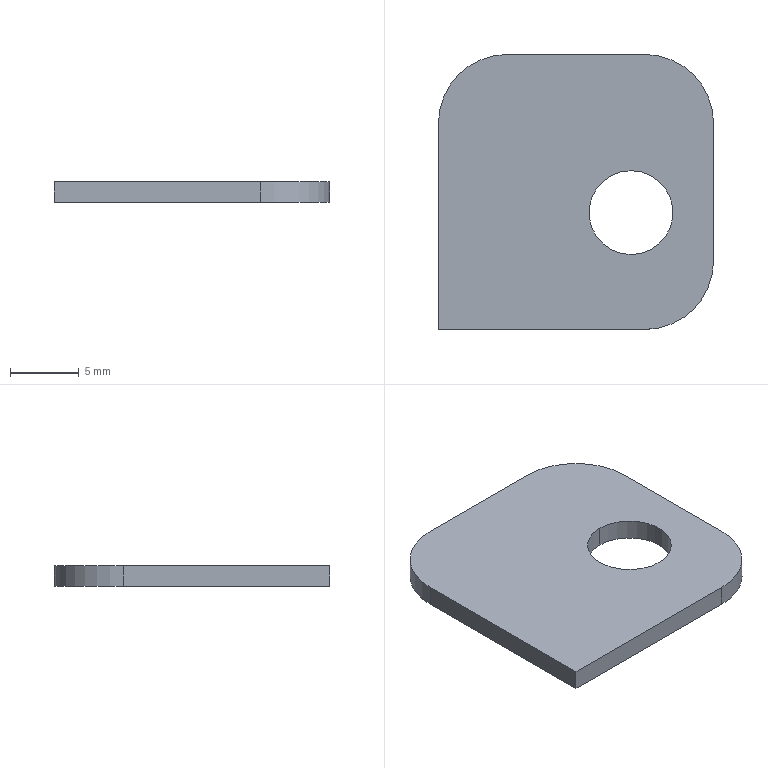Part | STEP file | 1 solid | 12 faces | box 20 x 20 x 1.5 mm | volume 532.02 mm3 | plane 7 | cylinder 5 | commonest cylinder face diameters 10 x3 6.1 x2
STEP:
#1=CARTESIAN_POINT('',(0.,0.,0.));
#2=DIRECTION('',(0.,0.,1.));
#3=DIRECTION('',(1.,0.,0.));
#4=AXIS2_PLACEMENT_3D('',#1,#2,#3);
#5=CARTESIAN_POINT('',(-500.773,4250.073,1738.644));
#6=VERTEX_POINT('',#5);
#7=CARTESIAN_POINT('',(-500.773,4256.573,1738.644));
#8=VERTEX_POINT('',#7);
#9=CARTESIAN_POINT('',(-500.773,4250.073,1738.644));
#10=DIRECTION('',(0.,1.,0.));
#11=VECTOR('',#10,1.);
#12=LINE('',#9,#11);
#13=CARTESIAN_POINT('',(-506.773,4250.073,1738.644));
#14=DIRECTION('',(0.,0.,-1.));
#15=DIRECTION('',(0.,-1.,0.));
#16=AXIS2_PLACEMENT_3D('',#13,#14,#15);
#17=PLANE('',#16);
#18=CARTESIAN_POINT('',(0.,-6.));
#19=DIRECTION('',(-1.,0.));
#20=VECTOR('',#19,1.);
#21=LINE('',#18,#20);
#22=(GEOMETRIC_REPRESENTATION_CONTEXT(2)PARAMETRIC_REPRESENTATION_CONTEXT()REPRESENTATION_CONTEXT('',''));
#23=DEFINITIONAL_REPRESENTATION('',(#21),#22);
#24=PCURVE('',#17,#23);
#25=CARTESIAN_POINT('',(-500.773,4255.823,1737.894));
#26=DIRECTION('',(-1.,0.,0.));
#27=DIRECTION('',(0.,-1.,0.));
#28=AXIS2_PLACEMENT_3D('',#25,#26,#27);
#29=PLANE('',#28);
#30=CARTESIAN_POINT('',(5.75,0.75));
#31=DIRECTION('',(-1.,0.));
#32=VECTOR('',#31,1.);
#33=LINE('',#30,#32);
#34=(GEOMETRIC_REPRESENTATION_CONTEXT(2)PARAMETRIC_REPRESENTATION_CONTEXT()REPRESENTATION_CONTEXT('',''));
#35=DEFINITIONAL_REPRESENTATION('',(#33),#34);
#36=PCURVE('',#29,#35);
#37=SURFACE_CURVE('',#12,(#24,#36),.PCURVE_S1.);
#38=EDGE_CURVE('',#6,#8,#37,.T.);
#39=ORIENTED_EDGE('',*,*,#38,.F.);
#40=CARTESIAN_POINT('',(-500.773,4246.573,1738.644));
#41=VERTEX_POINT('',#40);
#42=CARTESIAN_POINT('',(-500.773,4246.573,1738.644));
#43=DIRECTION('',(0.,1.,0.));
#44=VECTOR('',#43,1.);
#45=LINE('',#42,#44);
#46=CARTESIAN_POINT('',(3.5,-6.));
#47=DIRECTION('',(-1.,0.));
#48=VECTOR('',#47,1.);
#49=LINE('',#46,#48);
#50=(GEOMETRIC_REPRESENTATION_CONTEXT(2)PARAMETRIC_REPRESENTATION_CONTEXT()REPRESENTATION_CONTEXT('',''));
#51=DEFINITIONAL_REPRESENTATION('',(#49),#50);
#52=PCURVE('',#17,#51);
#53=CARTESIAN_POINT('',(-500.773,4245.823,1737.894));
#54=DIRECTION('',(-1.,0.,0.));
#55=DIRECTION('',(0.,-1.,0.));
#56=AXIS2_PLACEMENT_3D('',#53,#54,#55);
#57=PLANE('',#56);
#58=CARTESIAN_POINT('',(-0.75,0.75));
#59=DIRECTION('',(-1.,0.));
#60=VECTOR('',#59,1.);
#61=LINE('',#58,#60);
#62=(GEOMETRIC_REPRESENTATION_CONTEXT(2)PARAMETRIC_REPRESENTATION_CONTEXT()REPRESENTATION_CONTEXT('',''));
#63=DEFINITIONAL_REPRESENTATION('',(#61),#62);
#64=PCURVE('',#57,#63);
#65=SURFACE_CURVE('',#45,(#52,#64),.PCURVE_S1.);
#66=EDGE_CURVE('',#41,#6,#65,.T.);
#67=ORIENTED_EDGE('',*,*,#66,.F.);
#68=CARTESIAN_POINT('',(-505.773,4241.573,1738.644));
#69=VERTEX_POINT('',#68);
#70=CARTESIAN_POINT('',(-505.773,4246.573,1738.644));
#71=DIRECTION('',(0.,0.,1.));
#72=DIRECTION('',(0.,-1.,0.));
#73=AXIS2_PLACEMENT_3D('',#70,#71,#72);
#74=CIRCLE('',#73,5.);
#75=CARTESIAN_POINT('',(8.5,-1.));
#76=CARTESIAN_POINT('',(8.5,-9.66));
#77=CARTESIAN_POINT('',(1.,-5.33));
#78=CARTESIAN_POINT('',(-6.5,-1.));
#79=CARTESIAN_POINT('',(1.,3.33));
#80=CARTESIAN_POINT('',(8.5,7.66));
#81=CARTESIAN_POINT('',(8.5,-1.));
#82=(BOUNDED_CURVE()B_SPLINE_CURVE(2,(#75,#76,#77,#78,#79,#80,#81),.UNSPECIFIED.,.T.,.F.)B_SPLINE_CURVE_WITH_KNOTS((1,2,2,2,2,1),(-2.094,0.,2.094,4.189,6.283,8.378),.UNSPECIFIED.)CURVE()GEOMETRIC_REPRESENTATION_ITEM()RATIONAL_B_SPLINE_CURVE((1.,0.5,1.,0.5,1.,0.5,1.))REPRESENTATION_ITEM(''));
#83=(GEOMETRIC_REPRESENTATION_CONTEXT(2)PARAMETRIC_REPRESENTATION_CONTEXT()REPRESENTATION_CONTEXT('',''));
#84=DEFINITIONAL_REPRESENTATION('',(#82),#83);
#85=PCURVE('',#17,#84);
#86=CARTESIAN_POINT('',(-505.773,4246.573,1730.98));
#87=DIRECTION('',(0.,0.,1.));
#88=DIRECTION('',(-1.,0.,0.));
#89=AXIS2_PLACEMENT_3D('',#86,#87,#88);
#90=CYLINDRICAL_SURFACE('',#89,5.);
#91=CARTESIAN_POINT('',(1.571,7.664));
#92=DIRECTION('',(1.,0.));
#93=VECTOR('',#92,1.);
#94=LINE('',#91,#93);
#95=(GEOMETRIC_REPRESENTATION_CONTEXT(2)PARAMETRIC_REPRESENTATION_CONTEXT()REPRESENTATION_CONTEXT('',''));
#96=DEFINITIONAL_REPRESENTATION('',(#94),#95);
#97=PCURVE('',#90,#96);
#98=SURFACE_CURVE('',#74,(#85,#97),.PCURVE_S1.);
#99=EDGE_CURVE('',#69,#41,#98,.T.);
#100=ORIENTED_EDGE('',*,*,#99,.F.);
#101=CARTESIAN_POINT('',(-520.773,4241.573,1738.644));
#102=VERTEX_POINT('',#101);
#103=CARTESIAN_POINT('',(-520.773,4241.573,1738.644));
#104=DIRECTION('',(1.,0.,0.));
#105=VECTOR('',#104,1.);
#106=LINE('',#103,#105);
#107=CARTESIAN_POINT('',(8.5,14.));
#108=DIRECTION('',(0.,-1.));
#109=VECTOR('',#108,1.);
#110=LINE('',#107,#109);
#111=(GEOMETRIC_REPRESENTATION_CONTEXT(2)PARAMETRIC_REPRESENTATION_CONTEXT()REPRESENTATION_CONTEXT('',''));
#112=DEFINITIONAL_REPRESENTATION('',(#110),#111);
#113=PCURVE('',#17,#112);
#114=CARTESIAN_POINT('',(-510.773,4241.573,1737.894));
#115=DIRECTION('',(0.,1.,0.));
#116=DIRECTION('',(-1.,0.,0.));
#117=AXIS2_PLACEMENT_3D('',#114,#115,#116);
#118=PLANE('',#117);
#119=CARTESIAN_POINT('',(10.,0.75));
#120=DIRECTION('',(-1.,0.));
#121=VECTOR('',#120,1.);
#122=LINE('',#119,#121);
#123=(GEOMETRIC_REPRESENTATION_CONTEXT(2)PARAMETRIC_REPRESENTATION_CONTEXT()REPRESENTATION_CONTEXT('',''));
#124=DEFINITIONAL_REPRESENTATION('',(#122),#123);
#125=PCURVE('',#118,#124);
#126=SURFACE_CURVE('',#106,(#113,#125),.PCURVE_S1.);
#127=EDGE_CURVE('',#102,#69,#126,.T.);
#128=ORIENTED_EDGE('',*,*,#127,.F.);
#129=CARTESIAN_POINT('',(-520.773,4256.573,1738.644));
#130=VERTEX_POINT('',#129);
#131=CARTESIAN_POINT('',(-520.773,4256.573,1738.644));
#132=DIRECTION('',(0.,-1.,0.));
#133=VECTOR('',#132,1.);
#134=LINE('',#131,#133);
#135=CARTESIAN_POINT('',(-6.5,14.));
#136=DIRECTION('',(1.,0.));
#137=VECTOR('',#136,1.);
#138=LINE('',#135,#137);
#139=(GEOMETRIC_REPRESENTATION_CONTEXT(2)PARAMETRIC_REPRESENTATION_CONTEXT()REPRESENTATION_CONTEXT('',''));
#140=DEFINITIONAL_REPRESENTATION('',(#138),#139);
#141=PCURVE('',#17,#140);
#142=CARTESIAN_POINT('',(-520.773,4251.573,1737.894));
#143=DIRECTION('',(1.,0.,0.));
#144=DIRECTION('',(0.,1.,0.));
#145=AXIS2_PLACEMENT_3D('',#142,#143,#144);
#146=PLANE('',#145);
#147=CARTESIAN_POINT('',(5.,0.75));
#148=DIRECTION('',(-1.,0.));
#149=VECTOR('',#148,1.);
#150=LINE('',#147,#149);
#151=(GEOMETRIC_REPRESENTATION_CONTEXT(2)PARAMETRIC_REPRESENTATION_CONTEXT()REPRESENTATION_CONTEXT('',''));
#152=DEFINITIONAL_REPRESENTATION('',(#150),#151);
#153=PCURVE('',#146,#152);
#154=SURFACE_CURVE('',#134,(#141,#153),.PCURVE_S1.);
#155=EDGE_CURVE('',#130,#102,#154,.T.);
#156=ORIENTED_EDGE('',*,*,#155,.F.);
#157=CARTESIAN_POINT('',(-515.773,4261.573,1738.644));
#158=VERTEX_POINT('',#157);
#159=CARTESIAN_POINT('',(-515.773,4256.573,1738.644));
#160=DIRECTION('',(0.,0.,1.));
#161=DIRECTION('',(0.,1.,0.));
#162=AXIS2_PLACEMENT_3D('',#159,#160,#161);
#163=CIRCLE('',#162,5.);
#164=CARTESIAN_POINT('',(-11.5,9.));
#165=CARTESIAN_POINT('',(-11.5,17.66));
#166=CARTESIAN_POINT('',(-4.,13.33));
#167=CARTESIAN_POINT('',(3.5,9.));
#168=CARTESIAN_POINT('',(-4.,4.67));
#169=CARTESIAN_POINT('',(-11.5,0.3397));
#170=CARTESIAN_POINT('',(-11.5,9.));
#171=(BOUNDED_CURVE()B_SPLINE_CURVE(2,(#164,#165,#166,#167,#168,#169,#170),.UNSPECIFIED.,.T.,.F.)B_SPLINE_CURVE_WITH_KNOTS((1,2,2,2,2,1),(-2.094,0.,2.094,4.189,6.283,8.378),.UNSPECIFIED.)CURVE()GEOMETRIC_REPRESENTATION_ITEM()RATIONAL_B_SPLINE_CURVE((1.,0.5,1.,0.5,1.,0.5,1.))REPRESENTATION_ITEM(''));
#172=(GEOMETRIC_REPRESENTATION_CONTEXT(2)PARAMETRIC_REPRESENTATION_CONTEXT()REPRESENTATION_CONTEXT('',''));
#173=DEFINITIONAL_REPRESENTATION('',(#171),#172);
#174=PCURVE('',#17,#173);
#175=CARTESIAN_POINT('',(-515.773,4256.573,1730.98));
#176=DIRECTION('',(0.,0.,1.));
#177=DIRECTION('',(1.,0.,0.));
#178=AXIS2_PLACEMENT_3D('',#175,#176,#177);
#179=CYLINDRICAL_SURFACE('',#178,5.);
#180=CARTESIAN_POINT('',(1.571,7.664));
#181=DIRECTION('',(1.,0.));
#182=VECTOR('',#181,1.);
#183=LINE('',#180,#182);
#184=(GEOMETRIC_REPRESENTATION_CONTEXT(2)PARAMETRIC_REPRESENTATION_CONTEXT()REPRESENTATION_CONTEXT('',''));
#185=DEFINITIONAL_REPRESENTATION('',(#183),#184);
#186=PCURVE('',#179,#185);
#187=SURFACE_CURVE('',#163,(#174,#186),.PCURVE_S1.);
#188=EDGE_CURVE('',#158,#130,#187,.T.);
#189=ORIENTED_EDGE('',*,*,#188,.F.);
#190=CARTESIAN_POINT('',(-505.773,4261.573,1738.644));
#191=VERTEX_POINT('',#190);
#192=CARTESIAN_POINT('',(-505.773,4261.573,1738.644));
#193=DIRECTION('',(-1.,0.,0.));
#194=VECTOR('',#193,1.);
#195=LINE('',#192,#194);
#196=CARTESIAN_POINT('',(-11.5,-1.));
#197=DIRECTION('',(0.,1.));
#198=VECTOR('',#197,1.);
#199=LINE('',#196,#198);
#200=(GEOMETRIC_REPRESENTATION_CONTEXT(2)PARAMETRIC_REPRESENTATION_CONTEXT()REPRESENTATION_CONTEXT('',''));
#201=DEFINITIONAL_REPRESENTATION('',(#199),#200);
#202=PCURVE('',#17,#201);
#203=CARTESIAN_POINT('',(-510.773,4261.573,1737.894));
#204=DIRECTION('',(0.,-1.,0.));
#205=DIRECTION('',(1.,0.,0.));
#206=AXIS2_PLACEMENT_3D('',#203,#204,#205);
#207=PLANE('',#206);
#208=CARTESIAN_POINT('',(5.,0.75));
#209=DIRECTION('',(-1.,0.));
#210=VECTOR('',#209,1.);
#211=LINE('',#208,#210);
#212=(GEOMETRIC_REPRESENTATION_CONTEXT(2)PARAMETRIC_REPRESENTATION_CONTEXT()REPRESENTATION_CONTEXT('',''));
#213=DEFINITIONAL_REPRESENTATION('',(#211),#212);
#214=PCURVE('',#207,#213);
#215=SURFACE_CURVE('',#195,(#202,#214),.PCURVE_S1.);
#216=EDGE_CURVE('',#191,#158,#215,.T.);
#217=ORIENTED_EDGE('',*,*,#216,.F.);
#218=CARTESIAN_POINT('',(-505.773,4256.573,1738.644));
#219=DIRECTION('',(0.,0.,1.));
#220=DIRECTION('',(1.,0.,0.));
#221=AXIS2_PLACEMENT_3D('',#218,#219,#220);
#222=CIRCLE('',#221,5.);
#223=CARTESIAN_POINT('',(-6.5,-6.));
#224=CARTESIAN_POINT('',(-15.16,-6.));
#225=CARTESIAN_POINT('',(-10.83,1.5));
#226=CARTESIAN_POINT('',(-6.5,9.));
#227=CARTESIAN_POINT('',(-2.17,1.5));
#228=CARTESIAN_POINT('',(2.16,-6.));
#229=CARTESIAN_POINT('',(-6.5,-6.));
#230=(BOUNDED_CURVE()B_SPLINE_CURVE(2,(#223,#224,#225,#226,#227,#228,#229),.UNSPECIFIED.,.T.,.F.)B_SPLINE_CURVE_WITH_KNOTS((1,2,2,2,2,1),(-2.094,0.,2.094,4.189,6.283,8.378),.UNSPECIFIED.)CURVE()GEOMETRIC_REPRESENTATION_ITEM()RATIONAL_B_SPLINE_CURVE((1.,0.5,1.,0.5,1.,0.5,1.))REPRESENTATION_ITEM(''));
#231=(GEOMETRIC_REPRESENTATION_CONTEXT(2)PARAMETRIC_REPRESENTATION_CONTEXT()REPRESENTATION_CONTEXT('',''));
#232=DEFINITIONAL_REPRESENTATION('',(#230),#231);
#233=PCURVE('',#17,#232);
#234=CARTESIAN_POINT('',(-505.773,4256.573,1730.98));
#235=DIRECTION('',(0.,0.,1.));
#236=DIRECTION('',(0.,-1.,0.));
#237=AXIS2_PLACEMENT_3D('',#234,#235,#236);
#238=CYLINDRICAL_SURFACE('',#237,5.);
#239=CARTESIAN_POINT('',(1.571,7.664));
#240=DIRECTION('',(1.,0.));
#241=VECTOR('',#240,1.);
#242=LINE('',#239,#241);
#243=(GEOMETRIC_REPRESENTATION_CONTEXT(2)PARAMETRIC_REPRESENTATION_CONTEXT()REPRESENTATION_CONTEXT('',''));
#244=DEFINITIONAL_REPRESENTATION('',(#242),#243);
#245=PCURVE('',#238,#244);
#246=SURFACE_CURVE('',#222,(#233,#245),.PCURVE_S1.);
#247=EDGE_CURVE('',#8,#191,#246,.T.);
#248=ORIENTED_EDGE('',*,*,#247,.F.);
#249=EDGE_LOOP('',(#39,#67,#100,#128,#156,#189,#217,#248));
#250=FACE_BOUND('',#249,.F.);
#251=CARTESIAN_POINT('',(-506.773,4247.023,1738.644));
#252=VERTEX_POINT('',#251);
#253=CARTESIAN_POINT('',(-506.773,4253.123,1738.644));
#254=VERTEX_POINT('',#253);
#255=CARTESIAN_POINT('',(-506.773,4250.073,1738.644));
#256=DIRECTION('',(0.,0.,-1.));
#257=DIRECTION('',(0.,-1.,0.));
#258=AXIS2_PLACEMENT_3D('',#255,#256,#257);
#259=CIRCLE('',#258,3.05);
#260=CARTESIAN_POINT('',(0.,0.));
#261=DIRECTION('',(1.,0.));
#262=AXIS2_PLACEMENT_2D('',#260,#261);
#263=CIRCLE('',#262,3.05);
#264=(GEOMETRIC_REPRESENTATION_CONTEXT(2)PARAMETRIC_REPRESENTATION_CONTEXT()REPRESENTATION_CONTEXT('',''));
#265=DEFINITIONAL_REPRESENTATION('',(#263),#264);
#266=PCURVE('',#17,#265);
#267=CARTESIAN_POINT('',(-506.773,4250.073,1737.894));
#268=DIRECTION('',(0.,0.,1.));
#269=DIRECTION('',(0.,1.,0.));
#270=AXIS2_PLACEMENT_3D('',#267,#268,#269);
#271=CYLINDRICAL_SURFACE('',#270,3.05);
#272=CARTESIAN_POINT('',(3.142,0.75));
#273=DIRECTION('',(-1.,0.));
#274=VECTOR('',#273,1.);
#275=LINE('',#272,#274);
#276=(GEOMETRIC_REPRESENTATION_CONTEXT(2)PARAMETRIC_REPRESENTATION_CONTEXT()REPRESENTATION_CONTEXT('',''));
#277=DEFINITIONAL_REPRESENTATION('',(#275),#276);
#278=PCURVE('',#271,#277);
#279=SURFACE_CURVE('',#259,(#266,#278),.PCURVE_S1.);
#280=EDGE_CURVE('',#252,#254,#279,.T.);
#281=ORIENTED_EDGE('',*,*,#280,.F.);
#282=CARTESIAN_POINT('',(-506.773,4250.073,1738.644));
#283=DIRECTION('',(0.,0.,-1.));
#284=DIRECTION('',(0.,1.,0.));
#285=AXIS2_PLACEMENT_3D('',#282,#283,#284);
#286=CIRCLE('',#285,3.05);
#287=CARTESIAN_POINT('',(0.,0.));
#288=DIRECTION('',(-1.,0.));
#289=AXIS2_PLACEMENT_2D('',#287,#288);
#290=CIRCLE('',#289,3.05);
#291=(GEOMETRIC_REPRESENTATION_CONTEXT(2)PARAMETRIC_REPRESENTATION_CONTEXT()REPRESENTATION_CONTEXT('',''));
#292=DEFINITIONAL_REPRESENTATION('',(#290),#291);
#293=PCURVE('',#17,#292);
#294=CARTESIAN_POINT('',(-506.773,4250.073,1737.894));
#295=DIRECTION('',(0.,0.,1.));
#296=DIRECTION('',(0.,-1.,0.));
#297=AXIS2_PLACEMENT_3D('',#294,#295,#296);
#298=CYLINDRICAL_SURFACE('',#297,3.05);
#299=CARTESIAN_POINT('',(3.142,0.75));
#300=DIRECTION('',(-1.,0.));
#301=VECTOR('',#300,1.);
#302=LINE('',#299,#301);
#303=(GEOMETRIC_REPRESENTATION_CONTEXT(2)PARAMETRIC_REPRESENTATION_CONTEXT()REPRESENTATION_CONTEXT('',''));
#304=DEFINITIONAL_REPRESENTATION('',(#302),#303);
#305=PCURVE('',#298,#304);
#306=SURFACE_CURVE('',#286,(#293,#305),.PCURVE_S1.);
#307=EDGE_CURVE('',#254,#252,#306,.T.);
#308=ORIENTED_EDGE('',*,*,#307,.F.);
#309=EDGE_LOOP('',(#281,#308));
#310=FACE_BOUND('',#309,.F.);
#311=ADVANCED_FACE('',(#250,#310),#17,.F.);
#312=CARTESIAN_POINT('',(-500.773,4250.073,1737.144));
#313=VERTEX_POINT('',#312);
#314=CARTESIAN_POINT('',(-500.773,4256.573,1737.144));
#315=VERTEX_POINT('',#314);
#316=CARTESIAN_POINT('',(-500.773,4250.073,1737.144));
#317=DIRECTION('',(0.,1.,0.));
#318=VECTOR('',#317,1.);
#319=LINE('',#316,#318);
#320=CARTESIAN_POINT('',(5.75,-0.75));
#321=DIRECTION('',(-1.,0.));
#322=VECTOR('',#321,1.);
#323=LINE('',#320,#322);
#324=(GEOMETRIC_REPRESENTATION_CONTEXT(2)PARAMETRIC_REPRESENTATION_CONTEXT()REPRESENTATION_CONTEXT('',''));
#325=DEFINITIONAL_REPRESENTATION('',(#323),#324);
#326=PCURVE('',#29,#325);
#327=CARTESIAN_POINT('',(-506.773,4250.073,1737.144));
#328=DIRECTION('',(0.,0.,-1.));
#329=DIRECTION('',(0.,-1.,0.));
#330=AXIS2_PLACEMENT_3D('',#327,#328,#329);
#331=PLANE('',#330);
#332=CARTESIAN_POINT('',(0.,-6.));
#333=DIRECTION('',(-1.,0.));
#334=VECTOR('',#333,1.);
#335=LINE('',#332,#334);
#336=(GEOMETRIC_REPRESENTATION_CONTEXT(2)PARAMETRIC_REPRESENTATION_CONTEXT()REPRESENTATION_CONTEXT('',''));
#337=DEFINITIONAL_REPRESENTATION('',(#335),#336);
#338=PCURVE('',#331,#337);
#339=SURFACE_CURVE('',#319,(#326,#338),.PCURVE_S1.);
#340=EDGE_CURVE('',#313,#315,#339,.T.);
#341=ORIENTED_EDGE('',*,*,#340,.F.);
#342=CARTESIAN_POINT('',(-500.773,4250.073,1738.644));
#343=DIRECTION('',(0.,0.,-1.));
#344=VECTOR('',#343,1.);
#345=LINE('',#342,#344);
#346=CARTESIAN_POINT('',(5.75,0.75));
#347=DIRECTION('',(0.,-1.));
#348=VECTOR('',#347,1.);
#349=LINE('',#346,#348);
#350=(GEOMETRIC_REPRESENTATION_CONTEXT(2)PARAMETRIC_REPRESENTATION_CONTEXT()REPRESENTATION_CONTEXT('',''));
#351=DEFINITIONAL_REPRESENTATION('',(#349),#350);
#352=PCURVE('',#29,#351);
#353=CARTESIAN_POINT('',(-4.25,0.75));
#354=DIRECTION('',(0.,-1.));
#355=VECTOR('',#354,1.);
#356=LINE('',#353,#355);
#357=(GEOMETRIC_REPRESENTATION_CONTEXT(2)PARAMETRIC_REPRESENTATION_CONTEXT()REPRESENTATION_CONTEXT('',''));
#358=DEFINITIONAL_REPRESENTATION('',(#356),#357);
#359=PCURVE('',#57,#358);
#360=SURFACE_CURVE('',#345,(#352,#359),.PCURVE_S1.);
#361=EDGE_CURVE('',#6,#313,#360,.T.);
#362=ORIENTED_EDGE('',*,*,#361,.F.);
#363=ORIENTED_EDGE('',*,*,#38,.T.);
#364=CARTESIAN_POINT('',(-500.773,4256.573,1738.644));
#365=DIRECTION('',(0.,0.,-1.));
#366=VECTOR('',#365,1.);
#367=LINE('',#364,#366);
#368=CARTESIAN_POINT('',(-0.75,0.75));
#369=DIRECTION('',(0.,-1.));
#370=VECTOR('',#369,1.);
#371=LINE('',#368,#370);
#372=(GEOMETRIC_REPRESENTATION_CONTEXT(2)PARAMETRIC_REPRESENTATION_CONTEXT()REPRESENTATION_CONTEXT('',''));
#373=DEFINITIONAL_REPRESENTATION('',(#371),#372);
#374=PCURVE('',#29,#373);
#375=CARTESIAN_POINT('',(1.571,7.664));
#376=DIRECTION('',(0.,-1.));
#377=VECTOR('',#376,1.);
#378=LINE('',#375,#377);
#379=(GEOMETRIC_REPRESENTATION_CONTEXT(2)PARAMETRIC_REPRESENTATION_CONTEXT()REPRESENTATION_CONTEXT('',''));
#380=DEFINITIONAL_REPRESENTATION('',(#378),#379);
#381=PCURVE('',#238,#380);
#382=SURFACE_CURVE('',#367,(#374,#381),.PCURVE_S1.);
#383=EDGE_CURVE('',#8,#315,#382,.T.);
#384=ORIENTED_EDGE('',*,*,#383,.T.);
#385=EDGE_LOOP('',(#341,#362,#363,#384));
#386=FACE_BOUND('',#385,.F.);
#387=ADVANCED_FACE('',(#386),#29,.F.);
#388=CARTESIAN_POINT('',(-505.773,4261.573,1737.144));
#389=VERTEX_POINT('',#388);
#390=CARTESIAN_POINT('',(-515.773,4261.573,1737.144));
#391=VERTEX_POINT('',#390);
#392=CARTESIAN_POINT('',(-505.773,4261.573,1737.144));
#393=DIRECTION('',(-1.,0.,0.));
#394=VECTOR('',#393,1.);
#395=LINE('',#392,#394);
#396=CARTESIAN_POINT('',(-11.5,-1.));
#397=DIRECTION('',(0.,1.));
#398=VECTOR('',#397,1.);
#399=LINE('',#396,#398);
#400=(GEOMETRIC_REPRESENTATION_CONTEXT(2)PARAMETRIC_REPRESENTATION_CONTEXT()REPRESENTATION_CONTEXT('',''));
#401=DEFINITIONAL_REPRESENTATION('',(#399),#400);
#402=PCURVE('',#331,#401);
#403=CARTESIAN_POINT('',(5.,-0.75));
#404=DIRECTION('',(-1.,0.));
#405=VECTOR('',#404,1.);
#406=LINE('',#403,#405);
#407=(GEOMETRIC_REPRESENTATION_CONTEXT(2)PARAMETRIC_REPRESENTATION_CONTEXT()REPRESENTATION_CONTEXT('',''));
#408=DEFINITIONAL_REPRESENTATION('',(#406),#407);
#409=PCURVE('',#207,#408);
#410=SURFACE_CURVE('',#395,(#402,#409),.PCURVE_S1.);
#411=EDGE_CURVE('',#389,#391,#410,.T.);
#412=ORIENTED_EDGE('',*,*,#411,.T.);
#413=CARTESIAN_POINT('',(-520.773,4256.573,1737.144));
#414=VERTEX_POINT('',#413);
#415=CARTESIAN_POINT('',(-515.773,4256.573,1737.144));
#416=DIRECTION('',(0.,0.,-1.));
#417=DIRECTION('',(-1.,0.,0.));
#418=AXIS2_PLACEMENT_3D('',#415,#416,#417);
#419=CIRCLE('',#418,5.);
#420=CARTESIAN_POINT('',(-6.5,9.));
#421=DIRECTION('',(0.,1.));
#422=AXIS2_PLACEMENT_2D('',#420,#421);
#423=CIRCLE('',#422,5.);
#424=(GEOMETRIC_REPRESENTATION_CONTEXT(2)PARAMETRIC_REPRESENTATION_CONTEXT()REPRESENTATION_CONTEXT('',''));
#425=DEFINITIONAL_REPRESENTATION('',(#423),#424);
#426=PCURVE('',#331,#425);
#427=CARTESIAN_POINT('',(3.142,6.164));
#428=DIRECTION('',(-1.,0.));
#429=VECTOR('',#428,1.);
#430=LINE('',#427,#429);
#431=(GEOMETRIC_REPRESENTATION_CONTEXT(2)PARAMETRIC_REPRESENTATION_CONTEXT()REPRESENTATION_CONTEXT('',''));
#432=DEFINITIONAL_REPRESENTATION('',(#430),#431);
#433=PCURVE('',#179,#432);
#434=SURFACE_CURVE('',#419,(#426,#433),.PCURVE_S1.);
#435=EDGE_CURVE('',#414,#391,#434,.T.);
#436=ORIENTED_EDGE('',*,*,#435,.F.);
#437=CARTESIAN_POINT('',(-520.773,4241.573,1737.144));
#438=VERTEX_POINT('',#437);
#439=CARTESIAN_POINT('',(-520.773,4256.573,1737.144));
#440=DIRECTION('',(0.,-1.,0.));
#441=VECTOR('',#440,1.);
#442=LINE('',#439,#441);
#443=CARTESIAN_POINT('',(-6.5,14.));
#444=DIRECTION('',(1.,0.));
#445=VECTOR('',#444,1.);
#446=LINE('',#443,#445);
#447=(GEOMETRIC_REPRESENTATION_CONTEXT(2)PARAMETRIC_REPRESENTATION_CONTEXT()REPRESENTATION_CONTEXT('',''));
#448=DEFINITIONAL_REPRESENTATION('',(#446),#447);
#449=PCURVE('',#331,#448);
#450=CARTESIAN_POINT('',(5.,-0.75));
#451=DIRECTION('',(-1.,0.));
#452=VECTOR('',#451,1.);
#453=LINE('',#450,#452);
#454=(GEOMETRIC_REPRESENTATION_CONTEXT(2)PARAMETRIC_REPRESENTATION_CONTEXT()REPRESENTATION_CONTEXT('',''));
#455=DEFINITIONAL_REPRESENTATION('',(#453),#454);
#456=PCURVE('',#146,#455);
#457=SURFACE_CURVE('',#442,(#449,#456),.PCURVE_S1.);
#458=EDGE_CURVE('',#414,#438,#457,.T.);
#459=ORIENTED_EDGE('',*,*,#458,.T.);
#460=CARTESIAN_POINT('',(-505.773,4241.573,1737.144));
#461=VERTEX_POINT('',#460);
#462=CARTESIAN_POINT('',(-520.773,4241.573,1737.144));
#463=DIRECTION('',(1.,0.,0.));
#464=VECTOR('',#463,1.);
#465=LINE('',#462,#464);
#466=CARTESIAN_POINT('',(8.5,14.));
#467=DIRECTION('',(0.,-1.));
#468=VECTOR('',#467,1.);
#469=LINE('',#466,#468);
#470=(GEOMETRIC_REPRESENTATION_CONTEXT(2)PARAMETRIC_REPRESENTATION_CONTEXT()REPRESENTATION_CONTEXT('',''));
#471=DEFINITIONAL_REPRESENTATION('',(#469),#470);
#472=PCURVE('',#331,#471);
#473=CARTESIAN_POINT('',(10.,-0.75));
#474=DIRECTION('',(-1.,0.));
#475=VECTOR('',#474,1.);
#476=LINE('',#473,#475);
#477=(GEOMETRIC_REPRESENTATION_CONTEXT(2)PARAMETRIC_REPRESENTATION_CONTEXT()REPRESENTATION_CONTEXT('',''));
#478=DEFINITIONAL_REPRESENTATION('',(#476),#477);
#479=PCURVE('',#118,#478);
#480=SURFACE_CURVE('',#465,(#472,#479),.PCURVE_S1.);
#481=EDGE_CURVE('',#438,#461,#480,.T.);
#482=ORIENTED_EDGE('',*,*,#481,.T.);
#483=CARTESIAN_POINT('',(-500.773,4246.573,1737.144));
#484=VERTEX_POINT('',#483);
#485=CARTESIAN_POINT('',(-505.773,4246.573,1737.144));
#486=DIRECTION('',(0.,0.,-1.));
#487=DIRECTION('',(1.,0.,0.));
#488=AXIS2_PLACEMENT_3D('',#485,#486,#487);
#489=CIRCLE('',#488,5.);
#490=CARTESIAN_POINT('',(3.5,-1.));
#491=DIRECTION('',(0.,-1.));
#492=AXIS2_PLACEMENT_2D('',#490,#491);
#493=CIRCLE('',#492,5.);
#494=(GEOMETRIC_REPRESENTATION_CONTEXT(2)PARAMETRIC_REPRESENTATION_CONTEXT()REPRESENTATION_CONTEXT('',''));
#495=DEFINITIONAL_REPRESENTATION('',(#493),#494);
#496=PCURVE('',#331,#495);
#497=CARTESIAN_POINT('',(3.142,6.164));
#498=DIRECTION('',(-1.,0.));
#499=VECTOR('',#498,1.);
#500=LINE('',#497,#499);
#501=(GEOMETRIC_REPRESENTATION_CONTEXT(2)PARAMETRIC_REPRESENTATION_CONTEXT()REPRESENTATION_CONTEXT('',''));
#502=DEFINITIONAL_REPRESENTATION('',(#500),#501);
#503=PCURVE('',#90,#502);
#504=SURFACE_CURVE('',#489,(#496,#503),.PCURVE_S1.);
#505=EDGE_CURVE('',#484,#461,#504,.T.);
#506=ORIENTED_EDGE('',*,*,#505,.F.);
#507=CARTESIAN_POINT('',(-500.773,4246.573,1737.144));
#508=DIRECTION('',(0.,1.,0.));
#509=VECTOR('',#508,1.);
#510=LINE('',#507,#509);
#511=CARTESIAN_POINT('',(3.5,-6.));
#512=DIRECTION('',(-1.,0.));
#513=VECTOR('',#512,1.);
#514=LINE('',#511,#513);
#515=(GEOMETRIC_REPRESENTATION_CONTEXT(2)PARAMETRIC_REPRESENTATION_CONTEXT()REPRESENTATION_CONTEXT('',''));
#516=DEFINITIONAL_REPRESENTATION('',(#514),#515);
#517=PCURVE('',#331,#516);
#518=CARTESIAN_POINT('',(-0.75,-0.75));
#519=DIRECTION('',(-1.,0.));
#520=VECTOR('',#519,1.);
#521=LINE('',#518,#520);
#522=(GEOMETRIC_REPRESENTATION_CONTEXT(2)PARAMETRIC_REPRESENTATION_CONTEXT()REPRESENTATION_CONTEXT('',''));
#523=DEFINITIONAL_REPRESENTATION('',(#521),#522);
#524=PCURVE('',#57,#523);
#525=SURFACE_CURVE('',#510,(#517,#524),.PCURVE_S1.);
#526=EDGE_CURVE('',#484,#313,#525,.T.);
#527=ORIENTED_EDGE('',*,*,#526,.T.);
#528=ORIENTED_EDGE('',*,*,#340,.T.);
#529=CARTESIAN_POINT('',(-505.773,4256.573,1737.144));
#530=DIRECTION('',(0.,0.,-1.));
#531=DIRECTION('',(0.,1.,0.));
#532=AXIS2_PLACEMENT_3D('',#529,#530,#531);
#533=CIRCLE('',#532,5.);
#534=CARTESIAN_POINT('',(-6.5,-1.));
#535=DIRECTION('',(-1.,0.));
#536=AXIS2_PLACEMENT_2D('',#534,#535);
#537=CIRCLE('',#536,5.);
#538=(GEOMETRIC_REPRESENTATION_CONTEXT(2)PARAMETRIC_REPRESENTATION_CONTEXT()REPRESENTATION_CONTEXT('',''));
#539=DEFINITIONAL_REPRESENTATION('',(#537),#538);
#540=PCURVE('',#331,#539);
#541=CARTESIAN_POINT('',(3.142,6.164));
#542=DIRECTION('',(-1.,0.));
#543=VECTOR('',#542,1.);
#544=LINE('',#541,#543);
#545=(GEOMETRIC_REPRESENTATION_CONTEXT(2)PARAMETRIC_REPRESENTATION_CONTEXT()REPRESENTATION_CONTEXT('',''));
#546=DEFINITIONAL_REPRESENTATION('',(#544),#545);
#547=PCURVE('',#238,#546);
#548=SURFACE_CURVE('',#533,(#540,#547),.PCURVE_S1.);
#549=EDGE_CURVE('',#389,#315,#548,.T.);
#550=ORIENTED_EDGE('',*,*,#549,.F.);
#551=EDGE_LOOP('',(#412,#436,#459,#482,#506,#527,#528,#550));
#552=FACE_BOUND('',#551,.F.);
#553=CARTESIAN_POINT('',(-506.773,4253.123,1737.144));
#554=VERTEX_POINT('',#553);
#555=CARTESIAN_POINT('',(-506.773,4247.023,1737.144));
#556=VERTEX_POINT('',#555);
#557=CARTESIAN_POINT('',(-506.773,4250.073,1737.144));
#558=DIRECTION('',(0.,0.,1.));
#559=DIRECTION('',(0.,1.,0.));
#560=AXIS2_PLACEMENT_3D('',#557,#558,#559);
#561=CIRCLE('',#560,3.05);
#562=CARTESIAN_POINT('',(-3.05,0.));
#563=CARTESIAN_POINT('',(-3.05,5.283));
#564=CARTESIAN_POINT('',(1.525,2.641));
#565=CARTESIAN_POINT('',(6.1,0.));
#566=CARTESIAN_POINT('',(1.525,-2.641));
#567=CARTESIAN_POINT('',(-3.05,-5.283));
#568=CARTESIAN_POINT('',(-3.05,0.));
#569=(BOUNDED_CURVE()B_SPLINE_CURVE(2,(#562,#563,#564,#565,#566,#567,#568),.UNSPECIFIED.,.T.,.F.)B_SPLINE_CURVE_WITH_KNOTS((1,2,2,2,2,1),(-2.094,0.,2.094,4.189,6.283,8.378),.UNSPECIFIED.)CURVE()GEOMETRIC_REPRESENTATION_ITEM()RATIONAL_B_SPLINE_CURVE((1.,0.5,1.,0.5,1.,0.5,1.))REPRESENTATION_ITEM(''));
#570=(GEOMETRIC_REPRESENTATION_CONTEXT(2)PARAMETRIC_REPRESENTATION_CONTEXT()REPRESENTATION_CONTEXT('',''));
#571=DEFINITIONAL_REPRESENTATION('',(#569),#570);
#572=PCURVE('',#331,#571);
#573=CARTESIAN_POINT('',(0.,-0.75));
#574=DIRECTION('',(1.,0.));
#575=VECTOR('',#574,1.);
#576=LINE('',#573,#575);
#577=(GEOMETRIC_REPRESENTATION_CONTEXT(2)PARAMETRIC_REPRESENTATION_CONTEXT()REPRESENTATION_CONTEXT('',''));
#578=DEFINITIONAL_REPRESENTATION('',(#576),#577);
#579=PCURVE('',#271,#578);
#580=SURFACE_CURVE('',#561,(#572,#579),.PCURVE_S1.);
#581=EDGE_CURVE('',#554,#556,#580,.T.);
#582=ORIENTED_EDGE('',*,*,#581,.F.);
#583=CARTESIAN_POINT('',(-506.773,4250.073,1737.144));
#584=DIRECTION('',(0.,0.,1.));
#585=DIRECTION('',(0.,-1.,0.));
#586=AXIS2_PLACEMENT_3D('',#583,#584,#585);
#587=CIRCLE('',#586,3.05);
#588=CARTESIAN_POINT('',(3.05,0.));
#589=CARTESIAN_POINT('',(3.05,-5.283));
#590=CARTESIAN_POINT('',(-1.525,-2.641));
#591=CARTESIAN_POINT('',(-6.1,0.));
#592=CARTESIAN_POINT('',(-1.525,2.641));
#593=CARTESIAN_POINT('',(3.05,5.283));
#594=CARTESIAN_POINT('',(3.05,0.));
#595=(BOUNDED_CURVE()B_SPLINE_CURVE(2,(#588,#589,#590,#591,#592,#593,#594),.UNSPECIFIED.,.T.,.F.)B_SPLINE_CURVE_WITH_KNOTS((1,2,2,2,2,1),(-2.094,0.,2.094,4.189,6.283,8.378),.UNSPECIFIED.)CURVE()GEOMETRIC_REPRESENTATION_ITEM()RATIONAL_B_SPLINE_CURVE((1.,0.5,1.,0.5,1.,0.5,1.))REPRESENTATION_ITEM(''));
#596=(GEOMETRIC_REPRESENTATION_CONTEXT(2)PARAMETRIC_REPRESENTATION_CONTEXT()REPRESENTATION_CONTEXT('',''));
#597=DEFINITIONAL_REPRESENTATION('',(#595),#596);
#598=PCURVE('',#331,#597);
#599=CARTESIAN_POINT('',(0.,-0.75));
#600=DIRECTION('',(1.,0.));
#601=VECTOR('',#600,1.);
#602=LINE('',#599,#601);
#603=(GEOMETRIC_REPRESENTATION_CONTEXT(2)PARAMETRIC_REPRESENTATION_CONTEXT()REPRESENTATION_CONTEXT('',''));
#604=DEFINITIONAL_REPRESENTATION('',(#602),#603);
#605=PCURVE('',#298,#604);
#606=SURFACE_CURVE('',#587,(#598,#605),.PCURVE_S1.);
#607=EDGE_CURVE('',#556,#554,#606,.T.);
#608=ORIENTED_EDGE('',*,*,#607,.F.);
#609=EDGE_LOOP('',(#582,#608));
#610=FACE_BOUND('',#609,.F.);
#611=ADVANCED_FACE('',(#552,#610),#331,.T.);
#612=ORIENTED_EDGE('',*,*,#216,.T.);
#613=CARTESIAN_POINT('',(-515.773,4261.573,1738.644));
#614=DIRECTION('',(0.,0.,-1.));
#615=VECTOR('',#614,1.);
#616=LINE('',#613,#615);
#617=CARTESIAN_POINT('',(-5.,0.75));
#618=DIRECTION('',(0.,-1.));
#619=VECTOR('',#618,1.);
#620=LINE('',#617,#619);
#621=(GEOMETRIC_REPRESENTATION_CONTEXT(2)PARAMETRIC_REPRESENTATION_CONTEXT()REPRESENTATION_CONTEXT('',''));
#622=DEFINITIONAL_REPRESENTATION('',(#620),#621);
#623=PCURVE('',#207,#622);
#624=CARTESIAN_POINT('',(1.571,7.664));
#625=DIRECTION('',(0.,-1.));
#626=VECTOR('',#625,1.);
#627=LINE('',#624,#626);
#628=(GEOMETRIC_REPRESENTATION_CONTEXT(2)PARAMETRIC_REPRESENTATION_CONTEXT()REPRESENTATION_CONTEXT('',''));
#629=DEFINITIONAL_REPRESENTATION('',(#627),#628);
#630=PCURVE('',#179,#629);
#631=SURFACE_CURVE('',#616,(#623,#630),.PCURVE_S1.);
#632=EDGE_CURVE('',#158,#391,#631,.T.);
#633=ORIENTED_EDGE('',*,*,#632,.T.);
#634=ORIENTED_EDGE('',*,*,#411,.F.);
#635=CARTESIAN_POINT('',(-505.773,4261.573,1737.144));
#636=DIRECTION('',(0.,0.,1.));
#637=VECTOR('',#636,1.);
#638=LINE('',#635,#637);
#639=CARTESIAN_POINT('',(5.,-0.75));
#640=DIRECTION('',(0.,1.));
#641=VECTOR('',#640,1.);
#642=LINE('',#639,#641);
#643=(GEOMETRIC_REPRESENTATION_CONTEXT(2)PARAMETRIC_REPRESENTATION_CONTEXT()REPRESENTATION_CONTEXT('',''));
#644=DEFINITIONAL_REPRESENTATION('',(#642),#643);
#645=PCURVE('',#207,#644);
#646=CARTESIAN_POINT('',(3.142,6.164));
#647=DIRECTION('',(0.,1.));
#648=VECTOR('',#647,1.);
#649=LINE('',#646,#648);
#650=(GEOMETRIC_REPRESENTATION_CONTEXT(2)PARAMETRIC_REPRESENTATION_CONTEXT()REPRESENTATION_CONTEXT('',''));
#651=DEFINITIONAL_REPRESENTATION('',(#649),#650);
#652=PCURVE('',#238,#651);
#653=SURFACE_CURVE('',#638,(#645,#652),.PCURVE_S1.);
#654=EDGE_CURVE('',#389,#191,#653,.T.);
#655=ORIENTED_EDGE('',*,*,#654,.T.);
#656=EDGE_LOOP('',(#612,#633,#634,#655));
#657=FACE_BOUND('',#656,.F.);
#658=ADVANCED_FACE('',(#657),#207,.F.);
#659=ORIENTED_EDGE('',*,*,#188,.F.);
#660=ORIENTED_EDGE('',*,*,#632,.T.);
#661=ORIENTED_EDGE('',*,*,#435,.F.);
#662=CARTESIAN_POINT('',(-520.773,4256.573,1737.144));
#663=DIRECTION('',(0.,0.,1.));
#664=VECTOR('',#663,1.);
#665=LINE('',#662,#664);
#666=CARTESIAN_POINT('',(3.142,6.164));
#667=DIRECTION('',(0.,1.));
#668=VECTOR('',#667,1.);
#669=LINE('',#666,#668);
#670=(GEOMETRIC_REPRESENTATION_CONTEXT(2)PARAMETRIC_REPRESENTATION_CONTEXT()REPRESENTATION_CONTEXT('',''));
#671=DEFINITIONAL_REPRESENTATION('',(#669),#670);
#672=PCURVE('',#179,#671);
#673=CARTESIAN_POINT('',(5.,-0.75));
#674=DIRECTION('',(0.,1.));
#675=VECTOR('',#674,1.);
#676=LINE('',#673,#675);
#677=(GEOMETRIC_REPRESENTATION_CONTEXT(2)PARAMETRIC_REPRESENTATION_CONTEXT()REPRESENTATION_CONTEXT('',''));
#678=DEFINITIONAL_REPRESENTATION('',(#676),#677);
#679=PCURVE('',#146,#678);
#680=SURFACE_CURVE('',#665,(#672,#679),.PCURVE_S1.);
#681=EDGE_CURVE('',#414,#130,#680,.T.);
#682=ORIENTED_EDGE('',*,*,#681,.T.);
#683=EDGE_LOOP('',(#659,#660,#661,#682));
#684=FACE_BOUND('',#683,.T.);
#685=ADVANCED_FACE('',(#684),#179,.T.);
#686=ORIENTED_EDGE('',*,*,#155,.T.);
#687=CARTESIAN_POINT('',(-520.773,4241.573,1738.644));
#688=DIRECTION('',(0.,0.,-1.));
#689=VECTOR('',#688,1.);
#690=LINE('',#687,#689);
#691=CARTESIAN_POINT('',(-10.,0.75));
#692=DIRECTION('',(0.,-1.));
#693=VECTOR('',#692,1.);
#694=LINE('',#691,#693);
#695=(GEOMETRIC_REPRESENTATION_CONTEXT(2)PARAMETRIC_REPRESENTATION_CONTEXT()REPRESENTATION_CONTEXT('',''));
#696=DEFINITIONAL_REPRESENTATION('',(#694),#695);
#697=PCURVE('',#146,#696);
#698=CARTESIAN_POINT('',(10.,0.75));
#699=DIRECTION('',(0.,-1.));
#700=VECTOR('',#699,1.);
#701=LINE('',#698,#700);
#702=(GEOMETRIC_REPRESENTATION_CONTEXT(2)PARAMETRIC_REPRESENTATION_CONTEXT()REPRESENTATION_CONTEXT('',''));
#703=DEFINITIONAL_REPRESENTATION('',(#701),#702);
#704=PCURVE('',#118,#703);
#705=SURFACE_CURVE('',#690,(#697,#704),.PCURVE_S1.);
#706=EDGE_CURVE('',#102,#438,#705,.T.);
#707=ORIENTED_EDGE('',*,*,#706,.T.);
#708=ORIENTED_EDGE('',*,*,#458,.F.);
#709=ORIENTED_EDGE('',*,*,#681,.T.);
#710=EDGE_LOOP('',(#686,#707,#708,#709));
#711=FACE_BOUND('',#710,.F.);
#712=ADVANCED_FACE('',(#711),#146,.F.);
#713=ORIENTED_EDGE('',*,*,#481,.F.);
#714=ORIENTED_EDGE('',*,*,#706,.F.);
#715=ORIENTED_EDGE('',*,*,#127,.T.);
#716=CARTESIAN_POINT('',(-505.773,4241.573,1738.644));
#717=DIRECTION('',(0.,0.,-1.));
#718=VECTOR('',#717,1.);
#719=LINE('',#716,#718);
#720=CARTESIAN_POINT('',(-5.,0.75));
#721=DIRECTION('',(0.,-1.));
#722=VECTOR('',#721,1.);
#723=LINE('',#720,#722);
#724=(GEOMETRIC_REPRESENTATION_CONTEXT(2)PARAMETRIC_REPRESENTATION_CONTEXT()REPRESENTATION_CONTEXT('',''));
#725=DEFINITIONAL_REPRESENTATION('',(#723),#724);
#726=PCURVE('',#118,#725);
#727=CARTESIAN_POINT('',(1.571,7.664));
#728=DIRECTION('',(0.,-1.));
#729=VECTOR('',#728,1.);
#730=LINE('',#727,#729);
#731=(GEOMETRIC_REPRESENTATION_CONTEXT(2)PARAMETRIC_REPRESENTATION_CONTEXT()REPRESENTATION_CONTEXT('',''));
#732=DEFINITIONAL_REPRESENTATION('',(#730),#731);
#733=PCURVE('',#90,#732);
#734=SURFACE_CURVE('',#719,(#726,#733),.PCURVE_S1.);
#735=EDGE_CURVE('',#69,#461,#734,.T.);
#736=ORIENTED_EDGE('',*,*,#735,.T.);
#737=EDGE_LOOP('',(#713,#714,#715,#736));
#738=FACE_BOUND('',#737,.F.);
#739=ADVANCED_FACE('',(#738),#118,.F.);
#740=ORIENTED_EDGE('',*,*,#99,.F.);
#741=ORIENTED_EDGE('',*,*,#735,.T.);
#742=ORIENTED_EDGE('',*,*,#505,.F.);
#743=CARTESIAN_POINT('',(-500.773,4246.573,1737.144));
#744=DIRECTION('',(0.,0.,1.));
#745=VECTOR('',#744,1.);
#746=LINE('',#743,#745);
#747=CARTESIAN_POINT('',(3.142,6.164));
#748=DIRECTION('',(0.,1.));
#749=VECTOR('',#748,1.);
#750=LINE('',#747,#749);
#751=(GEOMETRIC_REPRESENTATION_CONTEXT(2)PARAMETRIC_REPRESENTATION_CONTEXT()REPRESENTATION_CONTEXT('',''));
#752=DEFINITIONAL_REPRESENTATION('',(#750),#751);
#753=PCURVE('',#90,#752);
#754=CARTESIAN_POINT('',(-0.75,-0.75));
#755=DIRECTION('',(0.,1.));
#756=VECTOR('',#755,1.);
#757=LINE('',#754,#756);
#758=(GEOMETRIC_REPRESENTATION_CONTEXT(2)PARAMETRIC_REPRESENTATION_CONTEXT()REPRESENTATION_CONTEXT('',''));
#759=DEFINITIONAL_REPRESENTATION('',(#757),#758);
#760=PCURVE('',#57,#759);
#761=SURFACE_CURVE('',#746,(#753,#760),.PCURVE_S1.);
#762=EDGE_CURVE('',#484,#41,#761,.T.);
#763=ORIENTED_EDGE('',*,*,#762,.T.);
#764=EDGE_LOOP('',(#740,#741,#742,#763));
#765=FACE_BOUND('',#764,.T.);
#766=ADVANCED_FACE('',(#765),#90,.T.);
#767=ORIENTED_EDGE('',*,*,#66,.T.);
#768=ORIENTED_EDGE('',*,*,#361,.T.);
#769=ORIENTED_EDGE('',*,*,#526,.F.);
#770=ORIENTED_EDGE('',*,*,#762,.T.);
#771=EDGE_LOOP('',(#767,#768,#769,#770));
#772=FACE_BOUND('',#771,.F.);
#773=ADVANCED_FACE('',(#772),#57,.F.);
#774=ORIENTED_EDGE('',*,*,#247,.F.);
#775=ORIENTED_EDGE('',*,*,#383,.T.);
#776=ORIENTED_EDGE('',*,*,#549,.F.);
#777=ORIENTED_EDGE('',*,*,#654,.T.);
#778=EDGE_LOOP('',(#774,#775,#776,#777));
#779=FACE_BOUND('',#778,.T.);
#780=ADVANCED_FACE('',(#779),#238,.T.);
#781=CARTESIAN_POINT('',(-506.773,4253.123,1737.144));
#782=DIRECTION('',(0.,0.,1.));
#783=VECTOR('',#782,1.);
#784=LINE('',#781,#783);
#785=CARTESIAN_POINT('',(0.,-0.75));
#786=DIRECTION('',(0.,1.));
#787=VECTOR('',#786,1.);
#788=LINE('',#785,#787);
#789=(GEOMETRIC_REPRESENTATION_CONTEXT(2)PARAMETRIC_REPRESENTATION_CONTEXT()REPRESENTATION_CONTEXT('',''));
#790=DEFINITIONAL_REPRESENTATION('',(#788),#789);
#791=PCURVE('',#271,#790);
#792=CARTESIAN_POINT('',(3.142,-0.75));
#793=DIRECTION('',(0.,1.));
#794=VECTOR('',#793,1.);
#795=LINE('',#792,#794);
#796=(GEOMETRIC_REPRESENTATION_CONTEXT(2)PARAMETRIC_REPRESENTATION_CONTEXT()REPRESENTATION_CONTEXT('',''));
#797=DEFINITIONAL_REPRESENTATION('',(#795),#796);
#798=PCURVE('',#298,#797);
#799=SURFACE_CURVE('',#784,(#791,#798),.PCURVE_S1.);
#800=EDGE_CURVE('',#554,#254,#799,.T.);
#801=ORIENTED_EDGE('',*,*,#800,.F.);
#802=ORIENTED_EDGE('',*,*,#581,.T.);
#803=CARTESIAN_POINT('',(-506.773,4247.023,1737.144));
#804=DIRECTION('',(0.,0.,1.));
#805=VECTOR('',#804,1.);
#806=LINE('',#803,#805);
#807=CARTESIAN_POINT('',(3.142,-0.75));
#808=DIRECTION('',(0.,1.));
#809=VECTOR('',#808,1.);
#810=LINE('',#807,#809);
#811=(GEOMETRIC_REPRESENTATION_CONTEXT(2)PARAMETRIC_REPRESENTATION_CONTEXT()REPRESENTATION_CONTEXT('',''));
#812=DEFINITIONAL_REPRESENTATION('',(#810),#811);
#813=PCURVE('',#271,#812);
#814=CARTESIAN_POINT('',(0.,-0.75));
#815=DIRECTION('',(0.,1.));
#816=VECTOR('',#815,1.);
#817=LINE('',#814,#816);
#818=(GEOMETRIC_REPRESENTATION_CONTEXT(2)PARAMETRIC_REPRESENTATION_CONTEXT()REPRESENTATION_CONTEXT('',''));
#819=DEFINITIONAL_REPRESENTATION('',(#817),#818);
#820=PCURVE('',#298,#819);
#821=SURFACE_CURVE('',#806,(#813,#820),.PCURVE_S1.);
#822=EDGE_CURVE('',#556,#252,#821,.T.);
#823=ORIENTED_EDGE('',*,*,#822,.T.);
#824=ORIENTED_EDGE('',*,*,#280,.T.);
#825=EDGE_LOOP('',(#801,#802,#823,#824));
#826=FACE_BOUND('',#825,.F.);
#827=ADVANCED_FACE('',(#826),#271,.F.);
#828=ORIENTED_EDGE('',*,*,#822,.F.);
#829=ORIENTED_EDGE('',*,*,#607,.T.);
#830=ORIENTED_EDGE('',*,*,#800,.T.);
#831=ORIENTED_EDGE('',*,*,#307,.T.);
#832=EDGE_LOOP('',(#828,#829,#830,#831));
#833=FACE_BOUND('',#832,.F.);
#834=ADVANCED_FACE('',(#833),#298,.F.);
#835=CLOSED_SHELL('',(#311,#387,#611,#658,#685,#712,#739,#766,#773,#780,#827,#834));
#836=MANIFOLD_SOLID_BREP('',#835);
#837=(LENGTH_UNIT()NAMED_UNIT(*)SI_UNIT(.MILLI.,.METRE.));
#838=UNCERTAINTY_MEASURE_WITH_UNIT(LENGTH_MEASURE(0.0000001),#837,'','');
#839=(NAMED_UNIT(*)PLANE_ANGLE_UNIT()SI_UNIT($,.RADIAN.));
#840=(NAMED_UNIT(*)SI_UNIT($,.STERADIAN.)SOLID_ANGLE_UNIT());
#841=(GEOMETRIC_REPRESENTATION_CONTEXT(3)GLOBAL_UNCERTAINTY_ASSIGNED_CONTEXT((#838))GLOBAL_UNIT_ASSIGNED_CONTEXT((#837,#839,#840))REPRESENTATION_CONTEXT('',''));
#842=ADVANCED_BREP_SHAPE_REPRESENTATION('',(#4,#836),#841);